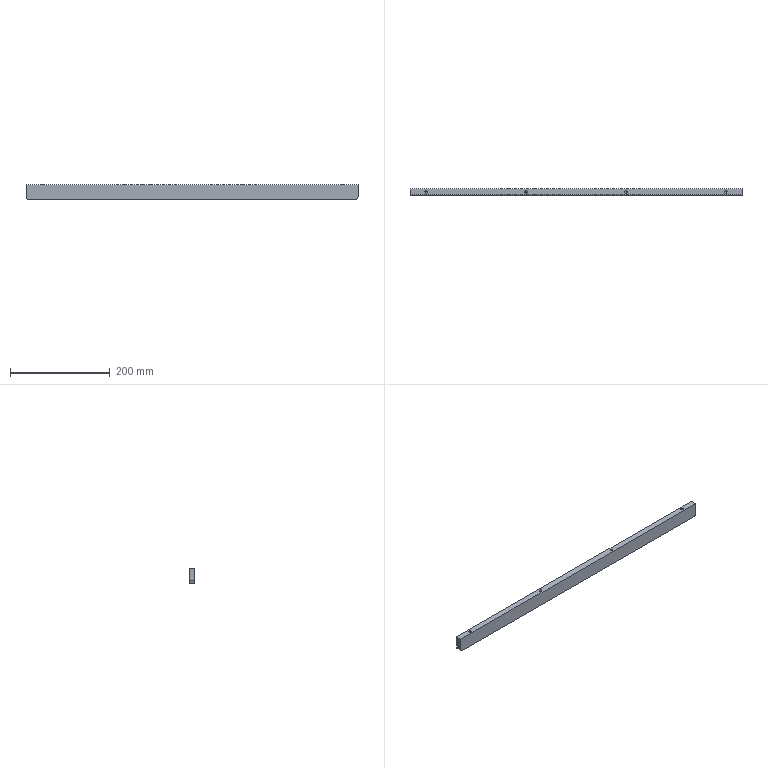Part | STEP file | 0-19-14 Reinforcing rib | 1 solid | 24 faces | box 665 x 12 x 30 mm | volume 237897 mm3 | cylinder 10 | cone 8 | plane 6 | commonest cylinder face diameters 5 x8 10 x2